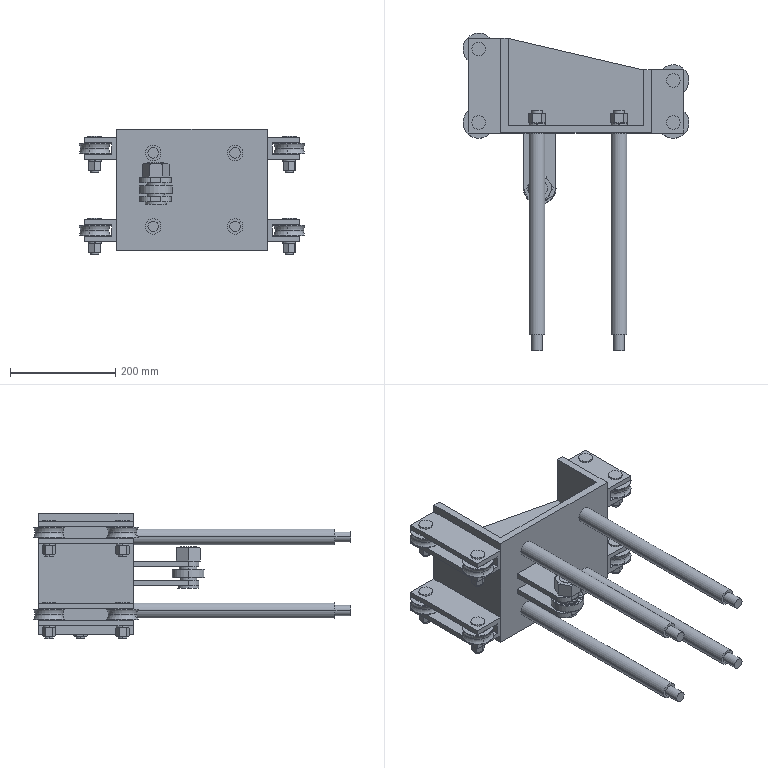Part | SolidWorks | features ReferencePattern 10, CompositeCurve 1, LocalSketchPattern 1, MirrorCompFeat 1 | 63 solids | 2096 faces | box 430 x 604 x 239 mm | volume 5255381 mm3 | plane 906 | cylinder 904 | cone 182 | torus 104 | commonest cylinder face diameters 6.5 x240 22.1 x88 35.1 x88 40 x38 9 x36 16 x32